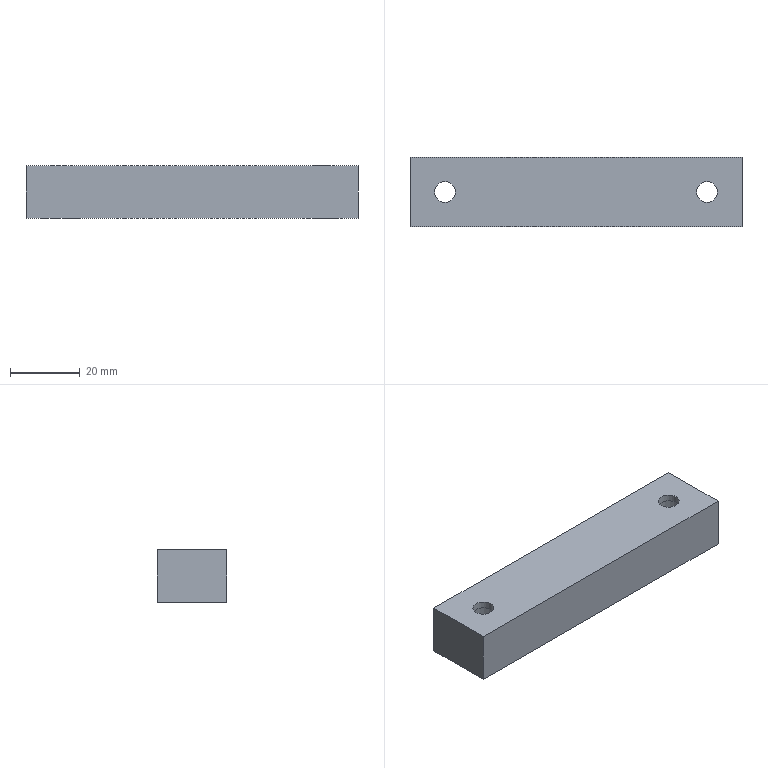Part | STEP file | gslz 2016.10.28-10_id2422_x_t | 1 solid | 12 faces | box 95 x 20 x 15 mm | volume 25916 mm3 | plane 8 | cylinder 4 | commonest cylinder face diameters 6 x2 11 x2
STEP:
#1=CARTESIAN_POINT('',(0.,0.,0.));
#2=DIRECTION('',(0.,0.,1.));
#3=DIRECTION('',(1.,0.,0.));
#4=AXIS2_PLACEMENT_3D('',#1,#2,#3);
#5=CARTESIAN_POINT('',(-873.5,250.,33.));
#6=VERTEX_POINT('',#5);
#7=CARTESIAN_POINT('',(-868.,250.,33.));
#8=DIRECTION('',(0.,0.,1.));
#9=DIRECTION('',(-1.,0.,0.));
#10=AXIS2_PLACEMENT_3D('',#7,#8,#9);
#11=CIRCLE('',#10,5.5);
#12=CARTESIAN_POINT('',(-868.,250.,35.));
#13=DIRECTION('',(0.,0.,-1.));
#14=DIRECTION('',(-1.,0.,0.));
#15=AXIS2_PLACEMENT_3D('',#12,#13,#14);
#16=CYLINDRICAL_SURFACE('',#15,5.5);
#17=CARTESIAN_POINT('',(6.283,2.));
#18=DIRECTION('',(-1.,0.));
#19=VECTOR('',#18,1.);
#20=LINE('',#17,#19);
#21=(GEOMETRIC_REPRESENTATION_CONTEXT(2)PARAMETRIC_REPRESENTATION_CONTEXT()REPRESENTATION_CONTEXT('',''));
#22=DEFINITIONAL_REPRESENTATION('',(#20),#21);
#23=PCURVE('',#16,#22);
#24=CARTESIAN_POINT('',(-830.5,250.,33.));
#25=DIRECTION('',(0.,0.,-1.));
#26=DIRECTION('',(1.,0.,0.));
#27=AXIS2_PLACEMENT_3D('',#24,#25,#26);
#28=PLANE('',#27);
#29=CARTESIAN_POINT('',(-43.,0.));
#30=CARTESIAN_POINT('',(-43.,9.526));
#31=CARTESIAN_POINT('',(-34.75,4.763));
#32=CARTESIAN_POINT('',(-26.5,0.));
#33=CARTESIAN_POINT('',(-34.75,-4.763));
#34=CARTESIAN_POINT('',(-43.,-9.526));
#35=CARTESIAN_POINT('',(-43.,0.));
#36=(BOUNDED_CURVE()B_SPLINE_CURVE(2,(#29,#30,#31,#32,#33,#34,#35),.UNSPECIFIED.,.T.,.F.)B_SPLINE_CURVE_WITH_KNOTS((1,2,2,2,2,1),(-2.094,0.,2.094,4.189,6.283,8.378),.UNSPECIFIED.)CURVE()GEOMETRIC_REPRESENTATION_ITEM()RATIONAL_B_SPLINE_CURVE((1.,0.5,1.,0.5,1.,0.5,1.))REPRESENTATION_ITEM(''));
#37=(GEOMETRIC_REPRESENTATION_CONTEXT(2)PARAMETRIC_REPRESENTATION_CONTEXT()REPRESENTATION_CONTEXT('',''));
#38=DEFINITIONAL_REPRESENTATION('',(#36),#37);
#39=PCURVE('',#28,#38);
#40=SURFACE_CURVE('',#11,(#23,#39),.PCURVE_S1.);
#41=EDGE_CURVE('',#6,#6,#40,.T.);
#42=ORIENTED_EDGE('',*,*,#41,.F.);
#43=CARTESIAN_POINT('',(-873.5,250.,20.));
#44=VERTEX_POINT('',#43);
#45=CARTESIAN_POINT('',(-873.5,250.,33.));
#46=CARTESIAN_POINT('',(-873.5,250.,20.));
#47=B_SPLINE_CURVE_WITH_KNOTS('',1,(#45,#46),.UNSPECIFIED.,.F.,.F.,(2,2),(2.,15.),.PIECEWISE_BEZIER_KNOTS.);
#48=CARTESIAN_POINT('',(6.283,0.));
#49=DIRECTION('',(0.,1.));
#50=VECTOR('',#49,1.);
#51=LINE('',#48,#50);
#52=(GEOMETRIC_REPRESENTATION_CONTEXT(2)PARAMETRIC_REPRESENTATION_CONTEXT()REPRESENTATION_CONTEXT('',''));
#53=DEFINITIONAL_REPRESENTATION('',(#51),#52);
#54=PCURVE('',#16,#53);
#55=CARTESIAN_POINT('',(0.,0.));
#56=DIRECTION('',(0.,1.));
#57=VECTOR('',#56,1.);
#58=LINE('',#55,#57);
#59=(GEOMETRIC_REPRESENTATION_CONTEXT(2)PARAMETRIC_REPRESENTATION_CONTEXT()REPRESENTATION_CONTEXT('',''));
#60=DEFINITIONAL_REPRESENTATION('',(#58),#59);
#61=PCURVE('',#16,#60);
#62=SEAM_CURVE('',#47,(#54,#61),.PCURVE_S1.);
#63=EDGE_CURVE('',#6,#44,#62,.T.);
#64=ORIENTED_EDGE('',*,*,#63,.T.);
#65=CARTESIAN_POINT('',(-862.5,250.,20.));
#66=VERTEX_POINT('',#65);
#67=CARTESIAN_POINT('',(-868.,250.,20.));
#68=DIRECTION('',(0.,0.,1.));
#69=DIRECTION('',(1.,0.,0.));
#70=AXIS2_PLACEMENT_3D('',#67,#68,#69);
#71=CIRCLE('',#70,5.5);
#72=CARTESIAN_POINT('',(9.425,15.));
#73=DIRECTION('',(-1.,0.));
#74=VECTOR('',#73,1.);
#75=LINE('',#72,#74);
#76=(GEOMETRIC_REPRESENTATION_CONTEXT(2)PARAMETRIC_REPRESENTATION_CONTEXT()REPRESENTATION_CONTEXT('',''));
#77=DEFINITIONAL_REPRESENTATION('',(#75),#76);
#78=PCURVE('',#16,#77);
#79=CARTESIAN_POINT('',(-885.5,250.,20.));
#80=DIRECTION('',(0.,0.,1.));
#81=DIRECTION('',(1.,0.,0.));
#82=AXIS2_PLACEMENT_3D('',#79,#80,#81);
#83=PLANE('',#82);
#84=CARTESIAN_POINT('',(17.5,0.));
#85=DIRECTION('',(1.,0.));
#86=AXIS2_PLACEMENT_2D('',#84,#85);
#87=CIRCLE('',#86,5.5);
#88=(GEOMETRIC_REPRESENTATION_CONTEXT(2)PARAMETRIC_REPRESENTATION_CONTEXT()REPRESENTATION_CONTEXT('',''));
#89=DEFINITIONAL_REPRESENTATION('',(#87),#88);
#90=PCURVE('',#83,#89);
#91=SURFACE_CURVE('',#71,(#78,#90),.PCURVE_S1.);
#92=EDGE_CURVE('',#44,#66,#91,.T.);
#93=ORIENTED_EDGE('',*,*,#92,.T.);
#94=CARTESIAN_POINT('',(-868.,250.,20.));
#95=DIRECTION('',(0.,0.,1.));
#96=DIRECTION('',(1.,0.,0.));
#97=AXIS2_PLACEMENT_3D('',#94,#95,#96);
#98=CIRCLE('',#97,5.5);
#99=CARTESIAN_POINT('',(3.142,15.));
#100=DIRECTION('',(-1.,0.));
#101=VECTOR('',#100,1.);
#102=LINE('',#99,#101);
#103=(GEOMETRIC_REPRESENTATION_CONTEXT(2)PARAMETRIC_REPRESENTATION_CONTEXT()REPRESENTATION_CONTEXT('',''));
#104=DEFINITIONAL_REPRESENTATION('',(#102),#103);
#105=PCURVE('',#16,#104);
#106=CARTESIAN_POINT('',(17.5,0.));
#107=DIRECTION('',(1.,0.));
#108=AXIS2_PLACEMENT_2D('',#106,#107);
#109=CIRCLE('',#108,5.5);
#110=(GEOMETRIC_REPRESENTATION_CONTEXT(2)PARAMETRIC_REPRESENTATION_CONTEXT()REPRESENTATION_CONTEXT('',''));
#111=DEFINITIONAL_REPRESENTATION('',(#109),#110);
#112=PCURVE('',#83,#111);
#113=SURFACE_CURVE('',#98,(#105,#112),.PCURVE_S1.);
#114=EDGE_CURVE('',#66,#44,#113,.T.);
#115=ORIENTED_EDGE('',*,*,#114,.T.);
#116=ORIENTED_EDGE('',*,*,#63,.F.);
#117=EDGE_LOOP('',(#42,#64,#93,#115,#116));
#118=FACE_BOUND('',#117,.F.);
#119=ADVANCED_FACE('',(#118),#16,.F.);
#120=CARTESIAN_POINT('',(-878.,260.,35.));
#121=VERTEX_POINT('',#120);
#122=CARTESIAN_POINT('',(-878.,260.,20.));
#123=VERTEX_POINT('',#122);
#124=CARTESIAN_POINT('',(-878.,260.,35.));
#125=DIRECTION('',(0.,0.,-1.));
#126=VECTOR('',#125,1.);
#127=LINE('',#124,#126);
#128=CARTESIAN_POINT('',(-765.5,260.,35.));
#129=DIRECTION('',(0.,-1.,0.));
#130=DIRECTION('',(0.,0.,-1.));
#131=AXIS2_PLACEMENT_3D('',#128,#129,#130);
#132=PLANE('',#131);
#133=CARTESIAN_POINT('',(0.,-112.5));
#134=DIRECTION('',(1.,0.));
#135=VECTOR('',#134,1.);
#136=LINE('',#133,#135);
#137=(GEOMETRIC_REPRESENTATION_CONTEXT(2)PARAMETRIC_REPRESENTATION_CONTEXT()REPRESENTATION_CONTEXT('',''));
#138=DEFINITIONAL_REPRESENTATION('',(#136),#137);
#139=PCURVE('',#132,#138);
#140=CARTESIAN_POINT('',(-878.,262.5,35.));
#141=DIRECTION('',(1.,0.,0.));
#142=DIRECTION('',(0.,0.,-1.));
#143=AXIS2_PLACEMENT_3D('',#140,#141,#142);
#144=PLANE('',#143);
#145=CARTESIAN_POINT('',(0.,-2.5));
#146=DIRECTION('',(1.,0.));
#147=VECTOR('',#146,1.);
#148=LINE('',#145,#147);
#149=(GEOMETRIC_REPRESENTATION_CONTEXT(2)PARAMETRIC_REPRESENTATION_CONTEXT()REPRESENTATION_CONTEXT('',''));
#150=DEFINITIONAL_REPRESENTATION('',(#148),#149);
#151=PCURVE('',#144,#150);
#152=SURFACE_CURVE('',#127,(#139,#151),.PCURVE_S1.);
#153=EDGE_CURVE('',#121,#123,#152,.T.);
#154=ORIENTED_EDGE('',*,*,#153,.F.);
#155=CARTESIAN_POINT('',(-783.,260.,35.));
#156=VERTEX_POINT('',#155);
#157=CARTESIAN_POINT('',(-885.5,260.,35.));
#158=DIRECTION('',(-1.,0.,0.));
#159=VECTOR('',#158,1.);
#160=LINE('',#157,#159);
#161=CARTESIAN_POINT('',(0.,-120.));
#162=DIRECTION('',(0.,-1.));
#163=VECTOR('',#162,1.);
#164=LINE('',#161,#163);
#165=(GEOMETRIC_REPRESENTATION_CONTEXT(2)PARAMETRIC_REPRESENTATION_CONTEXT()REPRESENTATION_CONTEXT('',''));
#166=DEFINITIONAL_REPRESENTATION('',(#164),#165);
#167=PCURVE('',#132,#166);
#168=CARTESIAN_POINT('',(-885.5,250.,35.));
#169=DIRECTION('',(0.,0.,1.));
#170=DIRECTION('',(1.,0.,0.));
#171=AXIS2_PLACEMENT_3D('',#168,#169,#170);
#172=PLANE('',#171);
#173=CARTESIAN_POINT('',(0.,10.));
#174=DIRECTION('',(-1.,0.));
#175=VECTOR('',#174,1.);
#176=LINE('',#173,#175);
#177=(GEOMETRIC_REPRESENTATION_CONTEXT(2)PARAMETRIC_REPRESENTATION_CONTEXT()REPRESENTATION_CONTEXT('',''));
#178=DEFINITIONAL_REPRESENTATION('',(#176),#177);
#179=PCURVE('',#172,#178);
#180=SURFACE_CURVE('',#160,(#167,#179),.PCURVE_S1.);
#181=EDGE_CURVE('',#156,#121,#180,.T.);
#182=ORIENTED_EDGE('',*,*,#181,.F.);
#183=CARTESIAN_POINT('',(-783.,260.,20.));
#184=VERTEX_POINT('',#183);
#185=CARTESIAN_POINT('',(-783.,260.,35.));
#186=DIRECTION('',(0.,0.,-1.));
#187=VECTOR('',#186,1.);
#188=LINE('',#185,#187);
#189=CARTESIAN_POINT('',(0.,-17.5));
#190=DIRECTION('',(1.,0.));
#191=VECTOR('',#190,1.);
#192=LINE('',#189,#191);
#193=(GEOMETRIC_REPRESENTATION_CONTEXT(2)PARAMETRIC_REPRESENTATION_CONTEXT()REPRESENTATION_CONTEXT('',''));
#194=DEFINITIONAL_REPRESENTATION('',(#192),#193);
#195=PCURVE('',#132,#194);
#196=CARTESIAN_POINT('',(-783.,237.5,35.));
#197=DIRECTION('',(-1.,0.,0.));
#198=DIRECTION('',(0.,0.,1.));
#199=AXIS2_PLACEMENT_3D('',#196,#197,#198);
#200=PLANE('',#199);
#201=CARTESIAN_POINT('',(0.,22.5));
#202=DIRECTION('',(-1.,0.));
#203=VECTOR('',#202,1.);
#204=LINE('',#201,#203);
#205=(GEOMETRIC_REPRESENTATION_CONTEXT(2)PARAMETRIC_REPRESENTATION_CONTEXT()REPRESENTATION_CONTEXT('',''));
#206=DEFINITIONAL_REPRESENTATION('',(#204),#205);
#207=PCURVE('',#200,#206);
#208=SURFACE_CURVE('',#188,(#195,#207),.PCURVE_S1.);
#209=EDGE_CURVE('',#156,#184,#208,.T.);
#210=ORIENTED_EDGE('',*,*,#209,.T.);
#211=CARTESIAN_POINT('',(-885.5,260.,20.));
#212=DIRECTION('',(-1.,0.,0.));
#213=VECTOR('',#212,1.);
#214=LINE('',#211,#213);
#215=CARTESIAN_POINT('',(15.,-120.));
#216=DIRECTION('',(0.,-1.));
#217=VECTOR('',#216,1.);
#218=LINE('',#215,#217);
#219=(GEOMETRIC_REPRESENTATION_CONTEXT(2)PARAMETRIC_REPRESENTATION_CONTEXT()REPRESENTATION_CONTEXT('',''));
#220=DEFINITIONAL_REPRESENTATION('',(#218),#219);
#221=PCURVE('',#132,#220);
#222=CARTESIAN_POINT('',(0.,10.));
#223=DIRECTION('',(-1.,0.));
#224=VECTOR('',#223,1.);
#225=LINE('',#222,#224);
#226=(GEOMETRIC_REPRESENTATION_CONTEXT(2)PARAMETRIC_REPRESENTATION_CONTEXT()REPRESENTATION_CONTEXT('',''));
#227=DEFINITIONAL_REPRESENTATION('',(#225),#226);
#228=PCURVE('',#83,#227);
#229=SURFACE_CURVE('',#214,(#221,#228),.PCURVE_S1.);
#230=EDGE_CURVE('',#184,#123,#229,.T.);
#231=ORIENTED_EDGE('',*,*,#230,.T.);
#232=EDGE_LOOP('',(#154,#182,#210,#231));
#233=FACE_BOUND('',#232,.T.);
#234=ADVANCED_FACE('',(#233),#132,.F.);
#235=ORIENTED_EDGE('',*,*,#209,.F.);
#236=CARTESIAN_POINT('',(-783.,240.,35.));
#237=VERTEX_POINT('',#236);
#238=CARTESIAN_POINT('',(-783.,237.5,35.));
#239=DIRECTION('',(0.,1.,0.));
#240=VECTOR('',#239,1.);
#241=LINE('',#238,#240);
#242=CARTESIAN_POINT('',(0.,0.));
#243=DIRECTION('',(0.,1.));
#244=VECTOR('',#243,1.);
#245=LINE('',#242,#244);
#246=(GEOMETRIC_REPRESENTATION_CONTEXT(2)PARAMETRIC_REPRESENTATION_CONTEXT()REPRESENTATION_CONTEXT('',''));
#247=DEFINITIONAL_REPRESENTATION('',(#245),#246);
#248=PCURVE('',#200,#247);
#249=CARTESIAN_POINT('',(102.5,-12.5));
#250=DIRECTION('',(0.,1.));
#251=VECTOR('',#250,1.);
#252=LINE('',#249,#251);
#253=(GEOMETRIC_REPRESENTATION_CONTEXT(2)PARAMETRIC_REPRESENTATION_CONTEXT()REPRESENTATION_CONTEXT('',''));
#254=DEFINITIONAL_REPRESENTATION('',(#252),#253);
#255=PCURVE('',#172,#254);
#256=SURFACE_CURVE('',#241,(#248,#255),.PCURVE_S1.);
#257=EDGE_CURVE('',#237,#156,#256,.T.);
#258=ORIENTED_EDGE('',*,*,#257,.F.);
#259=CARTESIAN_POINT('',(-783.,240.,20.));
#260=VERTEX_POINT('',#259);
#261=CARTESIAN_POINT('',(-783.,240.,35.));
#262=DIRECTION('',(0.,0.,-1.));
#263=VECTOR('',#262,1.);
#264=LINE('',#261,#263);
#265=CARTESIAN_POINT('',(0.,2.5));
#266=DIRECTION('',(-1.,0.));
#267=VECTOR('',#266,1.);
#268=LINE('',#265,#267);
#269=(GEOMETRIC_REPRESENTATION_CONTEXT(2)PARAMETRIC_REPRESENTATION_CONTEXT()REPRESENTATION_CONTEXT('',''));
#270=DEFINITIONAL_REPRESENTATION('',(#268),#269);
#271=PCURVE('',#200,#270);
#272=CARTESIAN_POINT('',(-895.5,240.,35.));
#273=DIRECTION('',(0.,1.,0.));
#274=DIRECTION('',(0.,0.,1.));
#275=AXIS2_PLACEMENT_3D('',#272,#273,#274);
#276=PLANE('',#275);
#277=CARTESIAN_POINT('',(0.,112.5));
#278=DIRECTION('',(-1.,0.));
#279=VECTOR('',#278,1.);
#280=LINE('',#277,#279);
#281=(GEOMETRIC_REPRESENTATION_CONTEXT(2)PARAMETRIC_REPRESENTATION_CONTEXT()REPRESENTATION_CONTEXT('',''));
#282=DEFINITIONAL_REPRESENTATION('',(#280),#281);
#283=PCURVE('',#276,#282);
#284=SURFACE_CURVE('',#264,(#271,#283),.PCURVE_S1.);
#285=EDGE_CURVE('',#237,#260,#284,.T.);
#286=ORIENTED_EDGE('',*,*,#285,.T.);
#287=CARTESIAN_POINT('',(-783.,237.5,20.));
#288=DIRECTION('',(0.,1.,0.));
#289=VECTOR('',#288,1.);
#290=LINE('',#287,#289);
#291=CARTESIAN_POINT('',(-15.,0.));
#292=DIRECTION('',(0.,1.));
#293=VECTOR('',#292,1.);
#294=LINE('',#291,#293);
#295=(GEOMETRIC_REPRESENTATION_CONTEXT(2)PARAMETRIC_REPRESENTATION_CONTEXT()REPRESENTATION_CONTEXT('',''));
#296=DEFINITIONAL_REPRESENTATION('',(#294),#295);
#297=PCURVE('',#200,#296);
#298=CARTESIAN_POINT('',(102.5,-12.5));
#299=DIRECTION('',(0.,1.));
#300=VECTOR('',#299,1.);
#301=LINE('',#298,#300);
#302=(GEOMETRIC_REPRESENTATION_CONTEXT(2)PARAMETRIC_REPRESENTATION_CONTEXT()REPRESENTATION_CONTEXT('',''));
#303=DEFINITIONAL_REPRESENTATION('',(#301),#302);
#304=PCURVE('',#83,#303);
#305=SURFACE_CURVE('',#290,(#297,#304),.PCURVE_S1.);
#306=EDGE_CURVE('',#260,#184,#305,.T.);
#307=ORIENTED_EDGE('',*,*,#306,.T.);
#308=EDGE_LOOP('',(#235,#258,#286,#307));
#309=FACE_BOUND('',#308,.T.);
#310=ADVANCED_FACE('',(#309),#200,.F.);
#311=ORIENTED_EDGE('',*,*,#285,.F.);
#312=CARTESIAN_POINT('',(-878.,240.,35.));
#313=VERTEX_POINT('',#312);
#314=CARTESIAN_POINT('',(-885.5,240.,35.));
#315=DIRECTION('',(1.,0.,0.));
#316=VECTOR('',#315,1.);
#317=LINE('',#314,#316);
#318=CARTESIAN_POINT('',(0.,10.));
#319=DIRECTION('',(0.,1.));
#320=VECTOR('',#319,1.);
#321=LINE('',#318,#320);
#322=(GEOMETRIC_REPRESENTATION_CONTEXT(2)PARAMETRIC_REPRESENTATION_CONTEXT()REPRESENTATION_CONTEXT('',''));
#323=DEFINITIONAL_REPRESENTATION('',(#321),#322);
#324=PCURVE('',#276,#323);
#325=CARTESIAN_POINT('',(0.,-10.));
#326=DIRECTION('',(1.,0.));
#327=VECTOR('',#326,1.);
#328=LINE('',#325,#327);
#329=(GEOMETRIC_REPRESENTATION_CONTEXT(2)PARAMETRIC_REPRESENTATION_CONTEXT()REPRESENTATION_CONTEXT('',''));
#330=DEFINITIONAL_REPRESENTATION('',(#328),#329);
#331=PCURVE('',#172,#330);
#332=SURFACE_CURVE('',#317,(#324,#331),.PCURVE_S1.);
#333=EDGE_CURVE('',#313,#237,#332,.T.);
#334=ORIENTED_EDGE('',*,*,#333,.F.);
#335=CARTESIAN_POINT('',(-878.,240.,20.));
#336=VERTEX_POINT('',#335);
#337=CARTESIAN_POINT('',(-878.,240.,35.));
#338=DIRECTION('',(0.,0.,-1.));
#339=VECTOR('',#338,1.);
#340=LINE('',#337,#339);
#341=CARTESIAN_POINT('',(0.,17.5));
#342=DIRECTION('',(-1.,0.));
#343=VECTOR('',#342,1.);
#344=LINE('',#341,#343);
#345=(GEOMETRIC_REPRESENTATION_CONTEXT(2)PARAMETRIC_REPRESENTATION_CONTEXT()REPRESENTATION_CONTEXT('',''));
#346=DEFINITIONAL_REPRESENTATION('',(#344),#345);
#347=PCURVE('',#276,#346);
#348=CARTESIAN_POINT('',(0.,-22.5));
#349=DIRECTION('',(1.,0.));
#350=VECTOR('',#349,1.);
#351=LINE('',#348,#350);
#352=(GEOMETRIC_REPRESENTATION_CONTEXT(2)PARAMETRIC_REPRESENTATION_CONTEXT()REPRESENTATION_CONTEXT('',''));
#353=DEFINITIONAL_REPRESENTATION('',(#351),#352);
#354=PCURVE('',#144,#353);
#355=SURFACE_CURVE('',#340,(#347,#354),.PCURVE_S1.);
#356=EDGE_CURVE('',#313,#336,#355,.T.);
#357=ORIENTED_EDGE('',*,*,#356,.T.);
#358=CARTESIAN_POINT('',(-885.5,240.,20.));
#359=DIRECTION('',(1.,0.,0.));
#360=VECTOR('',#359,1.);
#361=LINE('',#358,#360);
#362=CARTESIAN_POINT('',(-15.,10.));
#363=DIRECTION('',(0.,1.));
#364=VECTOR('',#363,1.);
#365=LINE('',#362,#364);
#366=(GEOMETRIC_REPRESENTATION_CONTEXT(2)PARAMETRIC_REPRESENTATION_CONTEXT()REPRESENTATION_CONTEXT('',''));
#367=DEFINITIONAL_REPRESENTATION('',(#365),#366);
#368=PCURVE('',#276,#367);
#369=CARTESIAN_POINT('',(0.,-10.));
#370=DIRECTION('',(1.,0.));
#371=VECTOR('',#370,1.);
#372=LINE('',#369,#371);
#373=(GEOMETRIC_REPRESENTATION_CONTEXT(2)PARAMETRIC_REPRESENTATION_CONTEXT()REPRESENTATION_CONTEXT('',''));
#374=DEFINITIONAL_REPRESENTATION('',(#372),#373);
#375=PCURVE('',#83,#374);
#376=SURFACE_CURVE('',#361,(#368,#375),.PCURVE_S1.);
#377=EDGE_CURVE('',#336,#260,#376,.T.);
#378=ORIENTED_EDGE('',*,*,#377,.T.);
#379=EDGE_LOOP('',(#311,#334,#357,#378));
#380=FACE_BOUND('',#379,.T.);
#381=ADVANCED_FACE('',(#380),#276,.F.);
#382=ORIENTED_EDGE('',*,*,#356,.F.);
#383=CARTESIAN_POINT('',(-878.,262.5,35.));
#384=DIRECTION('',(0.,-1.,0.));
#385=VECTOR('',#384,1.);
#386=LINE('',#383,#385);
#387=CARTESIAN_POINT('',(0.,0.));
#388=DIRECTION('',(0.,-1.));
#389=VECTOR('',#388,1.);
#390=LINE('',#387,#389);
#391=(GEOMETRIC_REPRESENTATION_CONTEXT(2)PARAMETRIC_REPRESENTATION_CONTEXT()REPRESENTATION_CONTEXT('',''));
#392=DEFINITIONAL_REPRESENTATION('',(#390),#391);
#393=PCURVE('',#144,#392);
#394=CARTESIAN_POINT('',(7.5,12.5));
#395=DIRECTION('',(0.,-1.));
#396=VECTOR('',#395,1.);
#397=LINE('',#394,#396);
#398=(GEOMETRIC_REPRESENTATION_CONTEXT(2)PARAMETRIC_REPRESENTATION_CONTEXT()REPRESENTATION_CONTEXT('',''));
#399=DEFINITIONAL_REPRESENTATION('',(#397),#398);
#400=PCURVE('',#172,#399);
#401=SURFACE_CURVE('',#386,(#393,#400),.PCURVE_S1.);
#402=EDGE_CURVE('',#121,#313,#401,.T.);
#403=ORIENTED_EDGE('',*,*,#402,.F.);
#404=ORIENTED_EDGE('',*,*,#153,.T.);
#405=CARTESIAN_POINT('',(-878.,262.5,20.));
#406=DIRECTION('',(0.,-1.,0.));
#407=VECTOR('',#406,1.);
#408=LINE('',#405,#407);
#409=CARTESIAN_POINT('',(15.,0.));
#410=DIRECTION('',(0.,-1.));
#411=VECTOR('',#410,1.);
#412=LINE('',#409,#411);
#413=(GEOMETRIC_REPRESENTATION_CONTEXT(2)PARAMETRIC_REPRESENTATION_CONTEXT()REPRESENTATION_CONTEXT('',''));
#414=DEFINITIONAL_REPRESENTATION('',(#412),#413);
#415=PCURVE('',#144,#414);
#416=CARTESIAN_POINT('',(7.5,12.5));
#417=DIRECTION('',(0.,-1.));
#418=VECTOR('',#417,1.);
#419=LINE('',#416,#418);
#420=(GEOMETRIC_REPRESENTATION_CONTEXT(2)PARAMETRIC_REPRESENTATION_CONTEXT()REPRESENTATION_CONTEXT('',''));
#421=DEFINITIONAL_REPRESENTATION('',(#419),#420);
#422=PCURVE('',#83,#421);
#423=SURFACE_CURVE('',#408,(#415,#422),.PCURVE_S1.);
#424=EDGE_CURVE('',#123,#336,#423,.T.);
#425=ORIENTED_EDGE('',*,*,#424,.T.);
#426=EDGE_LOOP('',(#382,#403,#404,#425));
#427=FACE_BOUND('',#426,.T.);
#428=ADVANCED_FACE('',(#427),#144,.F.);
#429=ORIENTED_EDGE('',*,*,#424,.F.);
#430=ORIENTED_EDGE('',*,*,#230,.F.);
#431=ORIENTED_EDGE('',*,*,#306,.F.);
#432=ORIENTED_EDGE('',*,*,#377,.F.);
#433=EDGE_LOOP('',(#429,#430,#431,#432));
#434=FACE_BOUND('',#433,.T.);
#435=ORIENTED_EDGE('',*,*,#114,.T.);
#436=ORIENTED_EDGE('',*,*,#92,.T.);
#437=EDGE_LOOP('',(#435,#436));
#438=FACE_BOUND('',#437,.T.);
#439=CARTESIAN_POINT('',(-787.5,250.,20.));
#440=VERTEX_POINT('',#439);
#441=CARTESIAN_POINT('',(-798.5,250.,20.));
#442=VERTEX_POINT('',#441);
#443=CARTESIAN_POINT('',(-793.,250.,20.));
#444=DIRECTION('',(0.,0.,1.));
#445=DIRECTION('',(1.,0.,0.));
#446=AXIS2_PLACEMENT_3D('',#443,#444,#445);
#447=CIRCLE('',#446,5.5);
#448=CARTESIAN_POINT('',(92.5,0.));
#449=DIRECTION('',(1.,0.));
#450=AXIS2_PLACEMENT_2D('',#448,#449);
#451=CIRCLE('',#450,5.5);
#452=(GEOMETRIC_REPRESENTATION_CONTEXT(2)PARAMETRIC_REPRESENTATION_CONTEXT()REPRESENTATION_CONTEXT('',''));
#453=DEFINITIONAL_REPRESENTATION('',(#451),#452);
#454=PCURVE('',#83,#453);
#455=CARTESIAN_POINT('',(-793.,250.,35.));
#456=DIRECTION('',(0.,0.,-1.));
#457=DIRECTION('',(-1.,0.,0.));
#458=AXIS2_PLACEMENT_3D('',#455,#456,#457);
#459=CYLINDRICAL_SURFACE('',#458,5.5);
#460=CARTESIAN_POINT('',(3.142,15.));
#461=DIRECTION('',(-1.,0.));
#462=VECTOR('',#461,1.);
#463=LINE('',#460,#462);
#464=(GEOMETRIC_REPRESENTATION_CONTEXT(2)PARAMETRIC_REPRESENTATION_CONTEXT()REPRESENTATION_CONTEXT('',''));
#465=DEFINITIONAL_REPRESENTATION('',(#463),#464);
#466=PCURVE('',#459,#465);
#467=SURFACE_CURVE('',#447,(#454,#466),.PCURVE_S1.);
#468=EDGE_CURVE('',#440,#442,#467,.T.);
#469=ORIENTED_EDGE('',*,*,#468,.T.);
#470=CARTESIAN_POINT('',(-793.,250.,20.));
#471=DIRECTION('',(0.,0.,1.));
#472=DIRECTION('',(1.,0.,0.));
#473=AXIS2_PLACEMENT_3D('',#470,#471,#472);
#474=CIRCLE('',#473,5.5);
#475=CARTESIAN_POINT('',(92.5,0.));
#476=DIRECTION('',(1.,0.));
#477=AXIS2_PLACEMENT_2D('',#475,#476);
#478=CIRCLE('',#477,5.5);
#479=(GEOMETRIC_REPRESENTATION_CONTEXT(2)PARAMETRIC_REPRESENTATION_CONTEXT()REPRESENTATION_CONTEXT('',''));
#480=DEFINITIONAL_REPRESENTATION('',(#478),#479);
#481=PCURVE('',#83,#480);
#482=CARTESIAN_POINT('',(9.425,15.));
#483=DIRECTION('',(-1.,0.));
#484=VECTOR('',#483,1.);
#485=LINE('',#482,#484);
#486=(GEOMETRIC_REPRESENTATION_CONTEXT(2)PARAMETRIC_REPRESENTATION_CONTEXT()REPRESENTATION_CONTEXT('',''));
#487=DEFINITIONAL_REPRESENTATION('',(#485),#486);
#488=PCURVE('',#459,#487);
#489=SURFACE_CURVE('',#474,(#481,#488),.PCURVE_S1.);
#490=EDGE_CURVE('',#442,#440,#489,.T.);
#491=ORIENTED_EDGE('',*,*,#490,.T.);
#492=EDGE_LOOP('',(#469,#491));
#493=FACE_BOUND('',#492,.T.);
#494=ADVANCED_FACE('',(#434,#438,#493),#83,.F.);
#495=CARTESIAN_POINT('',(-798.5,250.,33.));
#496=VERTEX_POINT('',#495);
#497=CARTESIAN_POINT('',(-793.,250.,33.));
#498=DIRECTION('',(0.,0.,1.));
#499=DIRECTION('',(-1.,0.,0.));
#500=AXIS2_PLACEMENT_3D('',#497,#498,#499);
#501=CIRCLE('',#500,5.5);
#502=CARTESIAN_POINT('',(6.283,2.));
#503=DIRECTION('',(-1.,0.));
#504=VECTOR('',#503,1.);
#505=LINE('',#502,#504);
#506=(GEOMETRIC_REPRESENTATION_CONTEXT(2)PARAMETRIC_REPRESENTATION_CONTEXT()REPRESENTATION_CONTEXT('',''));
#507=DEFINITIONAL_REPRESENTATION('',(#505),#506);
#508=PCURVE('',#459,#507);
#509=CARTESIAN_POINT('',(-830.5,250.,33.));
#510=DIRECTION('',(0.,0.,-1.));
#511=DIRECTION('',(1.,0.,0.));
#512=AXIS2_PLACEMENT_3D('',#509,#510,#511);
#513=PLANE('',#512);
#514=CARTESIAN_POINT('',(32.,0.));
#515=CARTESIAN_POINT('',(32.,9.526));
#516=CARTESIAN_POINT('',(40.25,4.763));
#517=CARTESIAN_POINT('',(48.5,0.));
#518=CARTESIAN_POINT('',(40.25,-4.763));
#519=CARTESIAN_POINT('',(32.,-9.526));
#520=CARTESIAN_POINT('',(32.,0.));
#521=(BOUNDED_CURVE()B_SPLINE_CURVE(2,(#514,#515,#516,#517,#518,#519,#520),.UNSPECIFIED.,.T.,.F.)B_SPLINE_CURVE_WITH_KNOTS((1,2,2,2,2,1),(-2.094,0.,2.094,4.189,6.283,8.378),.UNSPECIFIED.)CURVE()GEOMETRIC_REPRESENTATION_ITEM()RATIONAL_B_SPLINE_CURVE((1.,0.5,1.,0.5,1.,0.5,1.))REPRESENTATION_ITEM(''));
#522=(GEOMETRIC_REPRESENTATION_CONTEXT(2)PARAMETRIC_REPRESENTATION_CONTEXT()REPRESENTATION_CONTEXT('',''));
#523=DEFINITIONAL_REPRESENTATION('',(#521),#522);
#524=PCURVE('',#513,#523);
#525=SURFACE_CURVE('',#501,(#508,#524),.PCURVE_S1.);
#526=EDGE_CURVE('',#496,#496,#525,.T.);
#527=ORIENTED_EDGE('',*,*,#526,.F.);
#528=CARTESIAN_POINT('',(-798.5,250.,33.));
#529=CARTESIAN_POINT('',(-798.5,250.,20.));
#530=B_SPLINE_CURVE_WITH_KNOTS('',1,(#528,#529),.UNSPECIFIED.,.F.,.F.,(2,2),(2.,15.),.PIECEWISE_BEZIER_KNOTS.);
#531=CARTESIAN_POINT('',(6.283,0.));
#532=DIRECTION('',(0.,1.));
#533=VECTOR('',#532,1.);
#534=LINE('',#531,#533);
#535=(GEOMETRIC_REPRESENTATION_CONTEXT(2)PARAMETRIC_REPRESENTATION_CONTEXT()REPRESENTATION_CONTEXT('',''));
#536=DEFINITIONAL_REPRESENTATION('',(#534),#535);
#537=PCURVE('',#459,#536);
#538=CARTESIAN_POINT('',(0.,0.));
#539=DIRECTION('',(0.,1.));
#540=VECTOR('',#539,1.);
#541=LINE('',#538,#540);
#542=(GEOMETRIC_REPRESENTATION_CONTEXT(2)PARAMETRIC_REPRESENTATION_CONTEXT()REPRESENTATION_CONTEXT('',''));
#543=DEFINITIONAL_REPRESENTATION('',(#541),#542);
#544=PCURVE('',#459,#543);
#545=SEAM_CURVE('',#530,(#537,#544),.PCURVE_S1.);
#546=EDGE_CURVE('',#496,#442,#545,.T.);
#547=ORIENTED_EDGE('',*,*,#546,.T.);
#548=ORIENTED_EDGE('',*,*,#490,.T.);
#549=ORIENTED_EDGE('',*,*,#468,.T.);
#550=ORIENTED_EDGE('',*,*,#546,.F.);
#551=EDGE_LOOP('',(#527,#547,#548,#549,#550));
#552=FACE_BOUND('',#551,.F.);
#553=ADVANCED_FACE('',(#552),#459,.F.);
#554=CARTESIAN_POINT('',(-796.,250.,33.));
#555=VERTEX_POINT('',#554);
#556=CARTESIAN_POINT('',(-793.,250.,33.));
#557=DIRECTION('',(0.,0.,-1.));
#558=DIRECTION('',(-1.,0.,0.));
#559=AXIS2_PLACEMENT_3D('',#556,#557,#558);
#560=CIRCLE('',#559,3.);
#561=CARTESIAN_POINT('',(37.5,0.));
#562=DIRECTION('',(-1.,0.));
#563=AXIS2_PLACEMENT_2D('',#561,#562);
#564=CIRCLE('',#563,3.);
#565=(GEOMETRIC_REPRESENTATION_CONTEXT(2)PARAMETRIC_REPRESENTATION_CONTEXT()REPRESENTATION_CONTEXT('',''));
#566=DEFINITIONAL_REPRESENTATION('',(#564),#565);
#567=PCURVE('',#513,#566);
#568=CARTESIAN_POINT('',(-793.,250.,35.));
#569=DIRECTION('',(0.,0.,-1.));
#570=DIRECTION('',(-1.,0.,0.));
#571=AXIS2_PLACEMENT_3D('',#568,#569,#570);
#572=CYLINDRICAL_SURFACE('',#571,3.);
#573=CARTESIAN_POINT('',(0.,2.));
#574=DIRECTION('',(1.,0.));
#575=VECTOR('',#574,1.);
#576=LINE('',#573,#575);
#577=(GEOMETRIC_REPRESENTATION_CONTEXT(2)PARAMETRIC_REPRESENTATION_CONTEXT()REPRESENTATION_CONTEXT('',''));
#578=DEFINITIONAL_REPRESENTATION('',(#576),#577);
#579=PCURVE('',#572,#578);
#580=SURFACE_CURVE('',#560,(#567,#579),.PCURVE_S1.);
#581=EDGE_CURVE('',#555,#555,#580,.T.);
#582=ORIENTED_EDGE('',*,*,#581,.F.);
#583=EDGE_LOOP('',(#582));
#584=FACE_BOUND('',#583,.T.);
#585=ORIENTED_EDGE('',*,*,#526,.F.);
#586=EDGE_LOOP('',(#585));
#587=FACE_BOUND('',#586,.T.);
#588=ADVANCED_FACE('',(#584,#587),#513,.T.);
#589=CARTESIAN_POINT('',(-871.,250.,33.));
#590=VERTEX_POINT('',#589);
#591=CARTESIAN_POINT('',(-868.,250.,33.));
#592=DIRECTION('',(0.,0.,-1.));
#593=DIRECTION('',(-1.,0.,0.));
#594=AXIS2_PLACEMENT_3D('',#591,#592,#593);
#595=CIRCLE('',#594,3.);
#596=CARTESIAN_POINT('',(-37.5,0.));
#597=DIRECTION('',(-1.,0.));
#598=AXIS2_PLACEMENT_2D('',#596,#597);
#599=CIRCLE('',#598,3.);
#600=(GEOMETRIC_REPRESENTATION_CONTEXT(2)PARAMETRIC_REPRESENTATION_CONTEXT()REPRESENTATION_CONTEXT('',''));
#601=DEFINITIONAL_REPRESENTATION('',(#599),#600);
#602=PCURVE('',#28,#601);
#603=CARTESIAN_POINT('',(-868.,250.,35.));
#604=DIRECTION('',(0.,0.,-1.));
#605=DIRECTION('',(-1.,0.,0.));
#606=AXIS2_PLACEMENT_3D('',#603,#604,#605);
#607=CYLINDRICAL_SURFACE('',#606,3.);
#608=CARTESIAN_POINT('',(0.,2.));
#609=DIRECTION('',(1.,0.));
#610=VECTOR('',#609,1.);
#611=LINE('',#608,#610);
#612=(GEOMETRIC_REPRESENTATION_CONTEXT(2)PARAMETRIC_REPRESENTATION_CONTEXT()REPRESENTATION_CONTEXT('',''));
#613=DEFINITIONAL_REPRESENTATION('',(#611),#612);
#614=PCURVE('',#607,#613);
#615=SURFACE_CURVE('',#595,(#602,#614),.PCURVE_S1.);
#616=EDGE_CURVE('',#590,#590,#615,.T.);
#617=ORIENTED_EDGE('',*,*,#616,.F.);
#618=EDGE_LOOP('',(#617));
#619=FACE_BOUND('',#618,.T.);
#620=ORIENTED_EDGE('',*,*,#41,.F.);
#621=EDGE_LOOP('',(#620));
#622=FACE_BOUND('',#621,.T.);
#623=ADVANCED_FACE('',(#619,#622),#28,.T.);
#624=CARTESIAN_POINT('',(-871.,250.,35.));
#625=VERTEX_POINT('',#624);
#626=CARTESIAN_POINT('',(-865.,250.,35.));
#627=VERTEX_POINT('',#626);
#628=CARTESIAN_POINT('',(-868.,250.,35.));
#629=DIRECTION('',(0.,0.,1.));
#630=DIRECTION('',(1.,0.,0.));
#631=AXIS2_PLACEMENT_3D('',#628,#629,#630);
#632=CIRCLE('',#631,3.);
#633=CARTESIAN_POINT('',(9.425,0.));
#634=DIRECTION('',(-1.,0.));
#635=VECTOR('',#634,1.);
#636=LINE('',#633,#635);
#637=(GEOMETRIC_REPRESENTATION_CONTEXT(2)PARAMETRIC_REPRESENTATION_CONTEXT()REPRESENTATION_CONTEXT('',''));
#638=DEFINITIONAL_REPRESENTATION('',(#636),#637);
#639=PCURVE('',#607,#638);
#640=CARTESIAN_POINT('',(17.5,0.));
#641=DIRECTION('',(1.,0.));
#642=AXIS2_PLACEMENT_2D('',#640,#641);
#643=CIRCLE('',#642,3.);
#644=(GEOMETRIC_REPRESENTATION_CONTEXT(2)PARAMETRIC_REPRESENTATION_CONTEXT()REPRESENTATION_CONTEXT('',''));
#645=DEFINITIONAL_REPRESENTATION('',(#643),#644);
#646=PCURVE('',#172,#645);
#647=SURFACE_CURVE('',#632,(#639,#646),.PCURVE_S1.);
#648=EDGE_CURVE('',#625,#627,#647,.T.);
#649=ORIENTED_EDGE('',*,*,#648,.F.);
#650=CARTESIAN_POINT('',(-871.,250.,35.));
#651=CARTESIAN_POINT('',(-871.,250.,33.));
#652=B_SPLINE_CURVE_WITH_KNOTS('',1,(#650,#651),.UNSPECIFIED.,.F.,.F.,(2,2),(0.,2.),.PIECEWISE_BEZIER_KNOTS.);
#653=CARTESIAN_POINT('',(6.283,0.));
#654=DIRECTION('',(0.,1.));
#655=VECTOR('',#654,1.);
#656=LINE('',#653,#655);
#657=(GEOMETRIC_REPRESENTATION_CONTEXT(2)PARAMETRIC_REPRESENTATION_CONTEXT()REPRESENTATION_CONTEXT('',''));
#658=DEFINITIONAL_REPRESENTATION('',(#656),#657);
#659=PCURVE('',#607,#658);
#660=CARTESIAN_POINT('',(0.,0.));
#661=DIRECTION('',(0.,1.));
#662=VECTOR('',#661,1.);
#663=LINE('',#660,#662);
#664=(GEOMETRIC_REPRESENTATION_CONTEXT(2)PARAMETRIC_REPRESENTATION_CONTEXT()REPRESENTATION_CONTEXT('',''));
#665=DEFINITIONAL_REPRESENTATION('',(#663),#664);
#666=PCURVE('',#607,#665);
#667=SEAM_CURVE('',#652,(#659,#666),.PCURVE_S1.);
#668=EDGE_CURVE('',#625,#590,#667,.T.);
#669=ORIENTED_EDGE('',*,*,#668,.T.);
#670=ORIENTED_EDGE('',*,*,#616,.F.);
#671=ORIENTED_EDGE('',*,*,#668,.F.);
#672=CARTESIAN_POINT('',(-868.,250.,35.));
#673=DIRECTION('',(0.,0.,1.));
#674=DIRECTION('',(1.,0.,0.));
#675=AXIS2_PLACEMENT_3D('',#672,#673,#674);
#676=CIRCLE('',#675,3.);
#677=CARTESIAN_POINT('',(3.142,0.));
#678=DIRECTION('',(-1.,0.));
#679=VECTOR('',#678,1.);
#680=LINE('',#677,#679);
#681=(GEOMETRIC_REPRESENTATION_CONTEXT(2)PARAMETRIC_REPRESENTATION_CONTEXT()REPRESENTATION_CONTEXT('',''));
#682=DEFINITIONAL_REPRESENTATION('',(#680),#681);
#683=PCURVE('',#607,#682);
#684=CARTESIAN_POINT('',(17.5,0.));
#685=DIRECTION('',(1.,0.));
#686=AXIS2_PLACEMENT_2D('',#684,#685);
#687=CIRCLE('',#686,3.);
#688=(GEOMETRIC_REPRESENTATION_CONTEXT(2)PARAMETRIC_REPRESENTATION_CONTEXT()REPRESENTATION_CONTEXT('',''));
#689=DEFINITIONAL_REPRESENTATION('',(#687),#688);
#690=PCURVE('',#172,#689);
#691=SURFACE_CURVE('',#676,(#683,#690),.PCURVE_S1.);
#692=EDGE_CURVE('',#627,#625,#691,.T.);
#693=ORIENTED_EDGE('',*,*,#692,.F.);
#694=EDGE_LOOP('',(#649,#669,#670,#671,#693));
#695=FACE_BOUND('',#694,.F.);
#696=ADVANCED_FACE('',(#695),#607,.F.);
#697=CARTESIAN_POINT('',(-796.,250.,35.));
#698=VERTEX_POINT('',#697);
#699=CARTESIAN_POINT('',(-790.,250.,35.));
#700=VERTEX_POINT('',#699);
#701=CARTESIAN_POINT('',(-793.,250.,35.));
#702=DIRECTION('',(0.,0.,1.));
#703=DIRECTION('',(1.,0.,0.));
#704=AXIS2_PLACEMENT_3D('',#701,#702,#703);
#705=CIRCLE('',#704,3.);
#706=CARTESIAN_POINT('',(9.425,0.));
#707=DIRECTION('',(-1.,0.));
#708=VECTOR('',#707,1.);
#709=LINE('',#706,#708);
#710=(GEOMETRIC_REPRESENTATION_CONTEXT(2)PARAMETRIC_REPRESENTATION_CONTEXT()REPRESENTATION_CONTEXT('',''));
#711=DEFINITIONAL_REPRESENTATION('',(#709),#710);
#712=PCURVE('',#572,#711);
#713=CARTESIAN_POINT('',(92.5,0.));
#714=DIRECTION('',(1.,0.));
#715=AXIS2_PLACEMENT_2D('',#713,#714);
#716=CIRCLE('',#715,3.);
#717=(GEOMETRIC_REPRESENTATION_CONTEXT(2)PARAMETRIC_REPRESENTATION_CONTEXT()REPRESENTATION_CONTEXT('',''));
#718=DEFINITIONAL_REPRESENTATION('',(#716),#717);
#719=PCURVE('',#172,#718);
#720=SURFACE_CURVE('',#705,(#712,#719),.PCURVE_S1.);
#721=EDGE_CURVE('',#698,#700,#720,.T.);
#722=ORIENTED_EDGE('',*,*,#721,.F.);
#723=CARTESIAN_POINT('',(-796.,250.,35.));
#724=CARTESIAN_POINT('',(-796.,250.,33.));
#725=B_SPLINE_CURVE_WITH_KNOTS('',1,(#723,#724),.UNSPECIFIED.,.F.,.F.,(2,2),(0.,2.),.PIECEWISE_BEZIER_KNOTS.);
#726=CARTESIAN_POINT('',(6.283,0.));
#727=DIRECTION('',(0.,1.));
#728=VECTOR('',#727,1.);
#729=LINE('',#726,#728);
#730=(GEOMETRIC_REPRESENTATION_CONTEXT(2)PARAMETRIC_REPRESENTATION_CONTEXT()REPRESENTATION_CONTEXT('',''));
#731=DEFINITIONAL_REPRESENTATION('',(#729),#730);
#732=PCURVE('',#572,#731);
#733=CARTESIAN_POINT('',(0.,0.));
#734=DIRECTION('',(0.,1.));
#735=VECTOR('',#734,1.);
#736=LINE('',#733,#735);
#737=(GEOMETRIC_REPRESENTATION_CONTEXT(2)PARAMETRIC_REPRESENTATION_CONTEXT()REPRESENTATION_CONTEXT('',''));
#738=DEFINITIONAL_REPRESENTATION('',(#736),#737);
#739=PCURVE('',#572,#738);
#740=SEAM_CURVE('',#725,(#732,#739),.PCURVE_S1.);
#741=EDGE_CURVE('',#698,#555,#740,.T.);
#742=ORIENTED_EDGE('',*,*,#741,.T.);
#743=ORIENTED_EDGE('',*,*,#581,.F.);
#744=ORIENTED_EDGE('',*,*,#741,.F.);
#745=CARTESIAN_POINT('',(-793.,250.,35.));
#746=DIRECTION('',(0.,0.,1.));
#747=DIRECTION('',(1.,0.,0.));
#748=AXIS2_PLACEMENT_3D('',#745,#746,#747);
#749=CIRCLE('',#748,3.);
#750=CARTESIAN_POINT('',(3.142,0.));
#751=DIRECTION('',(-1.,0.));
#752=VECTOR('',#751,1.);
#753=LINE('',#750,#752);
#754=(GEOMETRIC_REPRESENTATION_CONTEXT(2)PARAMETRIC_REPRESENTATION_CONTEXT()REPRESENTATION_CONTEXT('',''));
#755=DEFINITIONAL_REPRESENTATION('',(#753),#754);
#756=PCURVE('',#572,#755);
#757=CARTESIAN_POINT('',(92.5,0.));
#758=DIRECTION('',(1.,0.));
#759=AXIS2_PLACEMENT_2D('',#757,#758);
#760=CIRCLE('',#759,3.);
#761=(GEOMETRIC_REPRESENTATION_CONTEXT(2)PARAMETRIC_REPRESENTATION_CONTEXT()REPRESENTATION_CONTEXT('',''));
#762=DEFINITIONAL_REPRESENTATION('',(#760),#761);
#763=PCURVE('',#172,#762);
#764=SURFACE_CURVE('',#749,(#756,#763),.PCURVE_S1.);
#765=EDGE_CURVE('',#700,#698,#764,.T.);
#766=ORIENTED_EDGE('',*,*,#765,.F.);
#767=EDGE_LOOP('',(#722,#742,#743,#744,#766));
#768=FACE_BOUND('',#767,.F.);
#769=ADVANCED_FACE('',(#768),#572,.F.);
#770=ORIENTED_EDGE('',*,*,#402,.T.);
#771=ORIENTED_EDGE('',*,*,#333,.T.);
#772=ORIENTED_EDGE('',*,*,#257,.T.);
#773=ORIENTED_EDGE('',*,*,#181,.T.);
#774=EDGE_LOOP('',(#770,#771,#772,#773));
#775=FACE_BOUND('',#774,.T.);
#776=ORIENTED_EDGE('',*,*,#692,.F.);
#777=ORIENTED_EDGE('',*,*,#648,.F.);
#778=EDGE_LOOP('',(#776,#777));
#779=FACE_BOUND('',#778,.T.);
#780=ORIENTED_EDGE('',*,*,#765,.F.);
#781=ORIENTED_EDGE('',*,*,#721,.F.);
#782=EDGE_LOOP('',(#780,#781));
#783=FACE_BOUND('',#782,.T.);
#784=ADVANCED_FACE('',(#775,#779,#783),#172,.T.);
#785=CLOSED_SHELL('',(#119,#234,#310,#381,#428,#494,#553,#588,#623,#696,#769,#784));
#786=MANIFOLD_SOLID_BREP('',#785);
#787=(LENGTH_UNIT()NAMED_UNIT(*)SI_UNIT(.MILLI.,.METRE.));
#788=UNCERTAINTY_MEASURE_WITH_UNIT(LENGTH_MEASURE(0.000002),#787,'','');
#789=(NAMED_UNIT(*)PLANE_ANGLE_UNIT()SI_UNIT($,.RADIAN.));
#790=(NAMED_UNIT(*)SI_UNIT($,.STERADIAN.)SOLID_ANGLE_UNIT());
#791=(GEOMETRIC_REPRESENTATION_CONTEXT(3)GLOBAL_UNCERTAINTY_ASSIGNED_CONTEXT((#788))GLOBAL_UNIT_ASSIGNED_CONTEXT((#787,#789,#790))REPRESENTATION_CONTEXT('',''));
#792=ADVANCED_BREP_SHAPE_REPRESENTATION('',(#4,#786),#791);